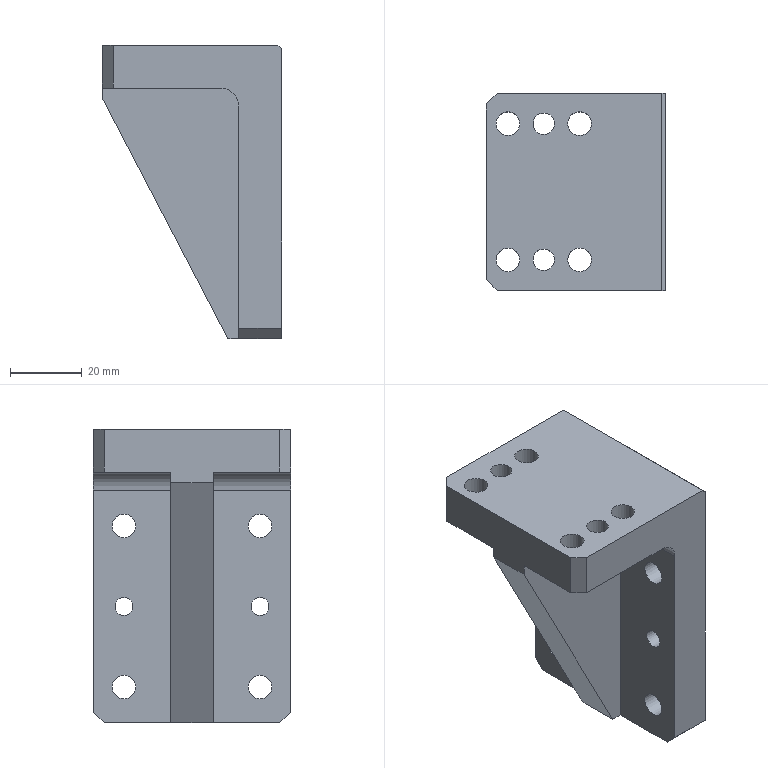Part | NX | 1 solid | 32 faces | box 50 x 55 x 82 mm | volume 92603 mm3 | plane 18 | cylinder 14 | commonest cylinder face diameters 6.6 x8 5 x2 6 x2 10 x2
STEP:
#1=CARTESIAN_POINT('',(24.,55.,41.));
#2=VERTEX_POINT('',#1);
#3=CARTESIAN_POINT('',(25.,55.,40.));
#4=VERTEX_POINT('',#3);
#5=CARTESIAN_POINT('',(25.,55.,40.));
#6=DIRECTION('',(0.7071,0.,-0.7071));
#7=VECTOR('',#6,1000.);
#8=LINE('',#5,#7);
#9=EDGE_CURVE('',#2,#4,#8,.T.);
#10=ORIENTED_EDGE('',*,*,#9,.F.);
#11=CARTESIAN_POINT('',(24.,0.,41.));
#12=VERTEX_POINT('',#11);
#13=CARTESIAN_POINT('',(24.,55.,41.));
#14=DIRECTION('',(0.,1.,0.));
#15=VECTOR('',#14,1000.);
#16=LINE('',#13,#15);
#17=EDGE_CURVE('',#12,#2,#16,.T.);
#18=ORIENTED_EDGE('',*,*,#17,.F.);
#19=CARTESIAN_POINT('',(25.,0.,40.));
#20=VERTEX_POINT('',#19);
#21=CARTESIAN_POINT('',(32.5,0.,32.5));
#22=DIRECTION('',(-0.7071,0.,0.7071));
#23=VECTOR('',#22,1000.);
#24=LINE('',#21,#23);
#25=EDGE_CURVE('',#20,#12,#24,.T.);
#26=ORIENTED_EDGE('',*,*,#25,.F.);
#27=CARTESIAN_POINT('',(25.,55.,40.));
#28=DIRECTION('',(0.,-1.,0.));
#29=VECTOR('',#28,1000.);
#30=LINE('',#27,#29);
#31=EDGE_CURVE('',#4,#20,#30,.T.);
#32=ORIENTED_EDGE('',*,*,#31,.F.);
#33=EDGE_LOOP('',(#10,#18,#26,#32));
#34=FACE_BOUND('',#33,.T.);
#35=CARTESIAN_POINT('',(25.,55.,40.));
#36=DIRECTION('',(-0.7071,0.,-0.7071));
#37=DIRECTION('',(0.,-1.,0.));
#38=AXIS2_PLACEMENT_3D('',#35,#36,#37);
#39=PLANE('',#38);
#40=ADVANCED_FACE('',(#34),#39,.F.);
#41=CARTESIAN_POINT('',(25.,52.,-41.));
#42=VERTEX_POINT('',#41);
#43=CARTESIAN_POINT('',(25.,55.,-38.));
#44=VERTEX_POINT('',#43);
#45=CARTESIAN_POINT('',(25.,55.,-38.));
#46=DIRECTION('',(0.,0.7071,0.7071));
#47=VECTOR('',#46,1000.);
#48=LINE('',#45,#47);
#49=EDGE_CURVE('',#42,#44,#48,.T.);
#50=ORIENTED_EDGE('',*,*,#49,.F.);
#51=CARTESIAN_POINT('',(13.,52.,-41.));
#52=VERTEX_POINT('',#51);
#53=CARTESIAN_POINT('',(-25.,52.,-41.));
#54=DIRECTION('',(1.,0.,0.));
#55=VECTOR('',#54,1000.);
#56=LINE('',#53,#55);
#57=EDGE_CURVE('',#52,#42,#56,.T.);
#58=ORIENTED_EDGE('',*,*,#57,.F.);
#59=CARTESIAN_POINT('',(13.,55.,-38.));
#60=VERTEX_POINT('',#59);
#61=CARTESIAN_POINT('',(13.,36.75,-56.25));
#62=DIRECTION('',(0.,-0.7071,-0.7071));
#63=VECTOR('',#62,1000.);
#64=LINE('',#61,#63);
#65=EDGE_CURVE('',#60,#52,#64,.T.);
#66=ORIENTED_EDGE('',*,*,#65,.F.);
#67=CARTESIAN_POINT('',(0.,55.,-38.));
#68=DIRECTION('',(-1.,0.,0.));
#69=VECTOR('',#68,1000.);
#70=LINE('',#67,#69);
#71=EDGE_CURVE('',#44,#60,#70,.T.);
#72=ORIENTED_EDGE('',*,*,#71,.F.);
#73=EDGE_LOOP('',(#50,#58,#66,#72));
#74=FACE_BOUND('',#73,.T.);
#75=CARTESIAN_POINT('',(0.,55.,-38.));
#76=DIRECTION('',(0.,-0.7071,0.7071));
#77=DIRECTION('',(-1.,0.,0.));
#78=AXIS2_PLACEMENT_3D('',#75,#76,#77);
#79=PLANE('',#78);
#80=ADVANCED_FACE('',(#74),#79,.F.);
#81=CARTESIAN_POINT('',(-25.,52.,29.));
#82=VERTEX_POINT('',#81);
#83=CARTESIAN_POINT('',(-22.,55.,29.));
#84=VERTEX_POINT('',#83);
#85=CARTESIAN_POINT('',(-21.25,55.75,29.));
#86=DIRECTION('',(0.7071,0.7071,0.));
#87=VECTOR('',#86,1000.);
#88=LINE('',#85,#87);
#89=EDGE_CURVE('',#82,#84,#88,.T.);
#90=ORIENTED_EDGE('',*,*,#89,.F.);
#91=CARTESIAN_POINT('',(-25.,52.,41.));
#92=VERTEX_POINT('',#91);
#93=CARTESIAN_POINT('',(-25.,52.,41.));
#94=DIRECTION('',(0.,0.,-1.));
#95=VECTOR('',#94,1000.);
#96=LINE('',#93,#95);
#97=EDGE_CURVE('',#92,#82,#96,.T.);
#98=ORIENTED_EDGE('',*,*,#97,.F.);
#99=CARTESIAN_POINT('',(-22.,55.,41.));
#100=VERTEX_POINT('',#99);
#101=CARTESIAN_POINT('',(-22.,55.,41.));
#102=DIRECTION('',(-0.7071,-0.7071,0.));
#103=VECTOR('',#102,1000.);
#104=LINE('',#101,#103);
#105=EDGE_CURVE('',#100,#92,#104,.T.);
#106=ORIENTED_EDGE('',*,*,#105,.F.);
#107=CARTESIAN_POINT('',(-22.,55.,0.));
#108=DIRECTION('',(0.,0.,1.));
#109=VECTOR('',#108,1000.);
#110=LINE('',#107,#109);
#111=EDGE_CURVE('',#84,#100,#110,.T.);
#112=ORIENTED_EDGE('',*,*,#111,.F.);
#113=EDGE_LOOP('',(#90,#98,#106,#112));
#114=FACE_BOUND('',#113,.T.);
#115=CARTESIAN_POINT('',(-22.,55.,0.));
#116=DIRECTION('',(0.7071,-0.7071,0.));
#117=DIRECTION('',(0.,0.,1.));
#118=AXIS2_PLACEMENT_3D('',#115,#116,#117);
#119=PLANE('',#118);
#120=ADVANCED_FACE('',(#114),#119,.F.);
#121=CARTESIAN_POINT('',(25.,0.,-38.));
#122=VERTEX_POINT('',#121);
#123=CARTESIAN_POINT('',(25.,3.,-41.));
#124=VERTEX_POINT('',#123);
#125=CARTESIAN_POINT('',(25.,3.,-41.));
#126=DIRECTION('',(0.,0.7071,-0.7071));
#127=VECTOR('',#126,1000.);
#128=LINE('',#125,#127);
#129=EDGE_CURVE('',#122,#124,#128,.T.);
#130=ORIENTED_EDGE('',*,*,#129,.F.);
#131=CARTESIAN_POINT('',(13.,0.,-38.));
#132=VERTEX_POINT('',#131);
#133=CARTESIAN_POINT('',(25.,0.,-38.));
#134=DIRECTION('',(1.,0.,0.));
#135=VECTOR('',#134,1000.);
#136=LINE('',#133,#135);
#137=EDGE_CURVE('',#132,#122,#136,.T.);
#138=ORIENTED_EDGE('',*,*,#137,.F.);
#139=CARTESIAN_POINT('',(13.,3.,-41.));
#140=VERTEX_POINT('',#139);
#141=CARTESIAN_POINT('',(13.,12.25,-50.25));
#142=DIRECTION('',(0.,-0.7071,0.7071));
#143=VECTOR('',#142,1000.);
#144=LINE('',#141,#143);
#145=EDGE_CURVE('',#140,#132,#144,.T.);
#146=ORIENTED_EDGE('',*,*,#145,.F.);
#147=CARTESIAN_POINT('',(13.,3.,-41.));
#148=DIRECTION('',(-1.,0.,0.));
#149=VECTOR('',#148,1000.);
#150=LINE('',#147,#149);
#151=EDGE_CURVE('',#124,#140,#150,.T.);
#152=ORIENTED_EDGE('',*,*,#151,.F.);
#153=EDGE_LOOP('',(#130,#138,#146,#152));
#154=FACE_BOUND('',#153,.T.);
#155=CARTESIAN_POINT('',(-25.,3.,-41.));
#156=DIRECTION('',(0.,-0.7071,-0.7071));
#157=DIRECTION('',(1.,0.,0.));
#158=AXIS2_PLACEMENT_3D('',#155,#156,#157);
#159=PLANE('',#158);
#160=ADVANCED_FACE('',(#154),#159,.T.);
#161=CARTESIAN_POINT('',(-22.,0.,29.));
#162=VERTEX_POINT('',#161);
#163=CARTESIAN_POINT('',(-25.,3.,29.));
#164=VERTEX_POINT('',#163);
#165=CARTESIAN_POINT('',(-15.25,-6.75,29.));
#166=DIRECTION('',(-0.7071,0.7071,0.));
#167=VECTOR('',#166,1000.);
#168=LINE('',#165,#167);
#169=EDGE_CURVE('',#162,#164,#168,.T.);
#170=ORIENTED_EDGE('',*,*,#169,.F.);
#171=CARTESIAN_POINT('',(-22.,0.,41.));
#172=VERTEX_POINT('',#171);
#173=CARTESIAN_POINT('',(-22.,0.,29.));
#174=DIRECTION('',(0.,0.,-1.));
#175=VECTOR('',#174,1000.);
#176=LINE('',#173,#175);
#177=EDGE_CURVE('',#172,#162,#176,.T.);
#178=ORIENTED_EDGE('',*,*,#177,.F.);
#179=CARTESIAN_POINT('',(-25.,3.,41.));
#180=VERTEX_POINT('',#179);
#181=CARTESIAN_POINT('',(-25.,3.,41.));
#182=DIRECTION('',(0.7071,-0.7071,0.));
#183=VECTOR('',#182,1000.);
#184=LINE('',#181,#183);
#185=EDGE_CURVE('',#180,#172,#184,.T.);
#186=ORIENTED_EDGE('',*,*,#185,.F.);
#187=CARTESIAN_POINT('',(-25.,3.,41.));
#188=DIRECTION('',(0.,0.,1.));
#189=VECTOR('',#188,1000.);
#190=LINE('',#187,#189);
#191=EDGE_CURVE('',#164,#180,#190,.T.);
#192=ORIENTED_EDGE('',*,*,#191,.F.);
#193=EDGE_LOOP('',(#170,#178,#186,#192));
#194=FACE_BOUND('',#193,.T.);
#195=CARTESIAN_POINT('',(-25.,3.,41.));
#196=DIRECTION('',(-0.7071,-0.7071,0.));
#197=DIRECTION('',(0.,0.,-1.));
#198=AXIS2_PLACEMENT_3D('',#195,#196,#197);
#199=PLANE('',#198);
#200=ADVANCED_FACE('',(#194),#199,.T.);
#201=CARTESIAN_POINT('',(8.,33.5,29.));
#202=VERTEX_POINT('',#201);
#203=CARTESIAN_POINT('',(13.,33.5,24.));
#204=VERTEX_POINT('',#203);
#205=CARTESIAN_POINT('',(8.,33.5,24.));
#206=DIRECTION('',(0.,1.,0.));
#207=DIRECTION('',(0.,0.,1.));
#208=AXIS2_PLACEMENT_3D('',#205,#206,#207);
#209=CIRCLE('',#208,5.);
#210=EDGE_CURVE('',#202,#204,#209,.T.);
#211=ORIENTED_EDGE('',*,*,#210,.F.);
#212=CARTESIAN_POINT('',(8.,55.,29.));
#213=VERTEX_POINT('',#212);
#214=CARTESIAN_POINT('',(8.,33.5,29.));
#215=DIRECTION('',(0.,-1.,0.));
#216=VECTOR('',#215,1000.);
#217=LINE('',#214,#216);
#218=EDGE_CURVE('',#213,#202,#217,.T.);
#219=ORIENTED_EDGE('',*,*,#218,.F.);
#220=CARTESIAN_POINT('',(13.,55.,24.));
#221=VERTEX_POINT('',#220);
#222=CARTESIAN_POINT('',(8.,55.,24.));
#223=DIRECTION('',(0.,-1.,0.));
#224=DIRECTION('',(0.,0.,-1.));
#225=AXIS2_PLACEMENT_3D('',#222,#223,#224);
#226=CIRCLE('',#225,5.);
#227=EDGE_CURVE('',#221,#213,#226,.T.);
#228=ORIENTED_EDGE('',*,*,#227,.F.);
#229=CARTESIAN_POINT('',(13.,33.5,24.));
#230=DIRECTION('',(0.,1.,0.));
#231=VECTOR('',#230,1000.);
#232=LINE('',#229,#231);
#233=EDGE_CURVE('',#204,#221,#232,.T.);
#234=ORIENTED_EDGE('',*,*,#233,.F.);
#235=EDGE_LOOP('',(#211,#219,#228,#234));
#236=FACE_BOUND('',#235,.T.);
#237=CARTESIAN_POINT('',(8.,33.5,24.));
#238=DIRECTION('',(0.,-1.,0.));
#239=DIRECTION('',(0.,0.,-1.));
#240=AXIS2_PLACEMENT_3D('',#237,#238,#239);
#241=CYLINDRICAL_SURFACE('',#240,5.);
#242=ADVANCED_FACE('',(#236),#241,.F.);
#243=CARTESIAN_POINT('',(13.,21.5,24.));
#244=VERTEX_POINT('',#243);
#245=CARTESIAN_POINT('',(8.,21.5,29.));
#246=VERTEX_POINT('',#245);
#247=CARTESIAN_POINT('',(8.,21.5,24.));
#248=DIRECTION('',(0.,-1.,0.));
#249=DIRECTION('',(0.,0.,-1.));
#250=AXIS2_PLACEMENT_3D('',#247,#248,#249);
#251=CIRCLE('',#250,5.);
#252=EDGE_CURVE('',#244,#246,#251,.T.);
#253=ORIENTED_EDGE('',*,*,#252,.F.);
#254=CARTESIAN_POINT('',(13.,0.,24.));
#255=VERTEX_POINT('',#254);
#256=CARTESIAN_POINT('',(13.,21.5,24.));
#257=DIRECTION('',(0.,1.,0.));
#258=VECTOR('',#257,1000.);
#259=LINE('',#256,#258);
#260=EDGE_CURVE('',#255,#244,#259,.T.);
#261=ORIENTED_EDGE('',*,*,#260,.F.);
#262=CARTESIAN_POINT('',(8.,0.,29.));
#263=VERTEX_POINT('',#262);
#264=CARTESIAN_POINT('',(8.,0.,24.));
#265=DIRECTION('',(0.,1.,0.));
#266=DIRECTION('',(0.,0.,-1.));
#267=AXIS2_PLACEMENT_3D('',#264,#265,#266);
#268=CIRCLE('',#267,5.);
#269=EDGE_CURVE('',#263,#255,#268,.T.);
#270=ORIENTED_EDGE('',*,*,#269,.F.);
#271=CARTESIAN_POINT('',(8.,0.,29.));
#272=DIRECTION('',(0.,-1.,0.));
#273=VECTOR('',#272,1000.);
#274=LINE('',#271,#273);
#275=EDGE_CURVE('',#246,#263,#274,.T.);
#276=ORIENTED_EDGE('',*,*,#275,.F.);
#277=EDGE_LOOP('',(#253,#261,#270,#276));
#278=FACE_BOUND('',#277,.T.);
#279=CARTESIAN_POINT('',(8.,21.5,24.));
#280=DIRECTION('',(0.,1.,0.));
#281=DIRECTION('',(0.,0.,1.));
#282=AXIS2_PLACEMENT_3D('',#279,#280,#281);
#283=CYLINDRICAL_SURFACE('',#282,5.);
#284=ADVANCED_FACE('',(#278),#283,.F.);
#285=CARTESIAN_POINT('',(13.,21.5,-41.));
#286=VERTEX_POINT('',#285);
#287=CARTESIAN_POINT('',(13.,21.5,-41.));
#288=DIRECTION('',(0.,0.,-1.));
#289=VECTOR('',#288,1000.);
#290=LINE('',#287,#289);
#291=EDGE_CURVE('',#244,#286,#290,.T.);
#292=ORIENTED_EDGE('',*,*,#291,.F.);
#293=ORIENTED_EDGE('',*,*,#252,.T.);
#294=CARTESIAN_POINT('',(-25.,21.5,29.));
#295=VERTEX_POINT('',#294);
#296=CARTESIAN_POINT('',(13.,21.5,29.));
#297=DIRECTION('',(1.,0.,0.));
#298=VECTOR('',#297,1000.);
#299=LINE('',#296,#298);
#300=EDGE_CURVE('',#295,#246,#299,.T.);
#301=ORIENTED_EDGE('',*,*,#300,.F.);
#302=CARTESIAN_POINT('',(-25.,21.5,26.));
#303=VERTEX_POINT('',#302);
#304=CARTESIAN_POINT('',(-25.,21.5,26.));
#305=DIRECTION('',(0.,0.,1.));
#306=VECTOR('',#305,1000.);
#307=LINE('',#304,#306);
#308=EDGE_CURVE('',#303,#295,#307,.T.);
#309=ORIENTED_EDGE('',*,*,#308,.F.);
#310=CARTESIAN_POINT('',(10.,21.5,-41.));
#311=VERTEX_POINT('',#310);
#312=CARTESIAN_POINT('',(-25.,21.5,26.));
#313=DIRECTION('',(-0.463,0.,0.8863));
#314=VECTOR('',#313,1000.);
#315=LINE('',#312,#314);
#316=EDGE_CURVE('',#311,#303,#315,.T.);
#317=ORIENTED_EDGE('',*,*,#316,.F.);
#318=CARTESIAN_POINT('',(13.,21.5,-41.));
#319=DIRECTION('',(-1.,0.,0.));
#320=VECTOR('',#319,1000.);
#321=LINE('',#318,#320);
#322=EDGE_CURVE('',#286,#311,#321,.T.);
#323=ORIENTED_EDGE('',*,*,#322,.F.);
#324=EDGE_LOOP('',(#292,#293,#301,#309,#317,#323));
#325=FACE_BOUND('',#324,.T.);
#326=CARTESIAN_POINT('',(0.,21.5,0.));
#327=DIRECTION('',(0.,-1.,0.));
#328=DIRECTION('',(0.,0.,1.));
#329=AXIS2_PLACEMENT_3D('',#326,#327,#328);
#330=PLANE('',#329);
#331=ADVANCED_FACE('',(#325),#330,.T.);
#332=CARTESIAN_POINT('',(13.,21.5,-41.));
#333=DIRECTION('',(0.,-1.,0.));
#334=VECTOR('',#333,1000.);
#335=LINE('',#332,#334);
#336=EDGE_CURVE('',#286,#140,#335,.T.);
#337=ORIENTED_EDGE('',*,*,#336,.T.);
#338=ORIENTED_EDGE('',*,*,#145,.T.);
#339=CARTESIAN_POINT('',(13.,0.,-41.));
#340=DIRECTION('',(0.,0.,-1.));
#341=VECTOR('',#340,1000.);
#342=LINE('',#339,#341);
#343=EDGE_CURVE('',#255,#132,#342,.T.);
#344=ORIENTED_EDGE('',*,*,#343,.F.);
#345=ORIENTED_EDGE('',*,*,#260,.T.);
#346=ORIENTED_EDGE('',*,*,#291,.T.);
#347=EDGE_LOOP('',(#337,#338,#344,#345,#346));
#348=FACE_BOUND('',#347,.T.);
#349=CARTESIAN_POINT('',(13.,8.5,17.3));
#350=VERTEX_POINT('',#349);
#351=CARTESIAN_POINT('',(13.,8.5,14.));
#352=DIRECTION('',(-1.,0.,0.));
#353=DIRECTION('',(0.,0.,1.));
#354=AXIS2_PLACEMENT_3D('',#351,#352,#353);
#355=CIRCLE('',#354,3.3);
#356=EDGE_CURVE('',#350,#350,#355,.T.);
#357=ORIENTED_EDGE('',*,*,#356,.F.);
#358=EDGE_LOOP('',(#357));
#359=FACE_BOUND('',#358,.T.);
#360=CARTESIAN_POINT('',(13.,8.5,-27.7));
#361=VERTEX_POINT('',#360);
#362=CARTESIAN_POINT('',(13.,8.5,-31.));
#363=DIRECTION('',(-1.,0.,0.));
#364=DIRECTION('',(0.,0.,1.));
#365=AXIS2_PLACEMENT_3D('',#362,#363,#364);
#366=CIRCLE('',#365,3.3);
#367=EDGE_CURVE('',#361,#361,#366,.T.);
#368=ORIENTED_EDGE('',*,*,#367,.F.);
#369=EDGE_LOOP('',(#368));
#370=FACE_BOUND('',#369,.T.);
#371=CARTESIAN_POINT('',(13.,8.5,-6.));
#372=VERTEX_POINT('',#371);
#373=CARTESIAN_POINT('',(13.,8.5,-8.5));
#374=DIRECTION('',(-1.,0.,0.));
#375=DIRECTION('',(0.,0.,1.));
#376=AXIS2_PLACEMENT_3D('',#373,#374,#375);
#377=CIRCLE('',#376,2.5);
#378=EDGE_CURVE('',#372,#372,#377,.T.);
#379=ORIENTED_EDGE('',*,*,#378,.F.);
#380=EDGE_LOOP('',(#379));
#381=FACE_BOUND('',#380,.T.);
#382=CARTESIAN_POINT('',(13.,21.5,-41.));
#383=DIRECTION('',(-1.,0.,0.));
#384=DIRECTION('',(0.,0.,1.));
#385=AXIS2_PLACEMENT_3D('',#382,#383,#384);
#386=PLANE('',#385);
#387=ADVANCED_FACE('',(#348,#359,#370,#381),#386,.T.);
#388=CARTESIAN_POINT('',(13.,0.,29.));
#389=DIRECTION('',(1.,0.,0.));
#390=VECTOR('',#389,1000.);
#391=LINE('',#388,#390);
#392=EDGE_CURVE('',#162,#263,#391,.T.);
#393=ORIENTED_EDGE('',*,*,#392,.F.);
#394=ORIENTED_EDGE('',*,*,#169,.T.);
#395=CARTESIAN_POINT('',(-25.,21.5,29.));
#396=DIRECTION('',(0.,-1.,0.));
#397=VECTOR('',#396,1000.);
#398=LINE('',#395,#397);
#399=EDGE_CURVE('',#295,#164,#398,.T.);
#400=ORIENTED_EDGE('',*,*,#399,.F.);
#401=ORIENTED_EDGE('',*,*,#300,.T.);
#402=ORIENTED_EDGE('',*,*,#275,.T.);
#403=EDGE_LOOP('',(#393,#394,#400,#401,#402));
#404=FACE_BOUND('',#403,.T.);
#405=CARTESIAN_POINT('',(-22.3,8.5,29.));
#406=VERTEX_POINT('',#405);
#407=CARTESIAN_POINT('',(-19.,8.5,29.));
#408=DIRECTION('',(0.,0.,-1.));
#409=DIRECTION('',(-1.,0.,0.));
#410=AXIS2_PLACEMENT_3D('',#407,#408,#409);
#411=CIRCLE('',#410,3.3);
#412=EDGE_CURVE('',#406,#406,#411,.T.);
#413=ORIENTED_EDGE('',*,*,#412,.F.);
#414=EDGE_LOOP('',(#413));
#415=FACE_BOUND('',#414,.T.);
#416=CARTESIAN_POINT('',(-2.3,8.5,29.));
#417=VERTEX_POINT('',#416);
#418=CARTESIAN_POINT('',(1.,8.5,29.));
#419=DIRECTION('',(0.,0.,-1.));
#420=DIRECTION('',(-1.,0.,0.));
#421=AXIS2_PLACEMENT_3D('',#418,#419,#420);
#422=CIRCLE('',#421,3.3);
#423=EDGE_CURVE('',#417,#417,#422,.T.);
#424=ORIENTED_EDGE('',*,*,#423,.F.);
#425=EDGE_LOOP('',(#424));
#426=FACE_BOUND('',#425,.T.);
#427=CARTESIAN_POINT('',(-12.,8.5,29.));
#428=VERTEX_POINT('',#427);
#429=CARTESIAN_POINT('',(-9.,8.5,29.));
#430=DIRECTION('',(0.,0.,-1.));
#431=DIRECTION('',(-1.,0.,0.));
#432=AXIS2_PLACEMENT_3D('',#429,#430,#431);
#433=CIRCLE('',#432,3.);
#434=EDGE_CURVE('',#428,#428,#433,.T.);
#435=ORIENTED_EDGE('',*,*,#434,.F.);
#436=EDGE_LOOP('',(#435));
#437=FACE_BOUND('',#436,.T.);
#438=CARTESIAN_POINT('',(13.,21.5,29.));
#439=DIRECTION('',(0.,0.,-1.));
#440=DIRECTION('',(-1.,0.,0.));
#441=AXIS2_PLACEMENT_3D('',#438,#439,#440);
#442=PLANE('',#441);
#443=ADVANCED_FACE('',(#404,#415,#426,#437),#442,.T.);
#444=CARTESIAN_POINT('',(-25.,33.5,29.));
#445=VERTEX_POINT('',#444);
#446=CARTESIAN_POINT('',(0.,33.5,29.));
#447=DIRECTION('',(1.,0.,0.));
#448=VECTOR('',#447,1000.);
#449=LINE('',#446,#448);
#450=EDGE_CURVE('',#445,#202,#449,.T.);
#451=ORIENTED_EDGE('',*,*,#450,.T.);
#452=ORIENTED_EDGE('',*,*,#210,.T.);
#453=CARTESIAN_POINT('',(13.,33.5,-41.));
#454=VERTEX_POINT('',#453);
#455=CARTESIAN_POINT('',(13.,33.5,0.));
#456=DIRECTION('',(0.,0.,-1.));
#457=VECTOR('',#456,1000.);
#458=LINE('',#455,#457);
#459=EDGE_CURVE('',#204,#454,#458,.T.);
#460=ORIENTED_EDGE('',*,*,#459,.T.);
#461=CARTESIAN_POINT('',(10.,33.5,-41.));
#462=VERTEX_POINT('',#461);
#463=CARTESIAN_POINT('',(13.,33.5,-41.));
#464=DIRECTION('',(-1.,0.,0.));
#465=VECTOR('',#464,1000.);
#466=LINE('',#463,#465);
#467=EDGE_CURVE('',#454,#462,#466,.T.);
#468=ORIENTED_EDGE('',*,*,#467,.T.);
#469=CARTESIAN_POINT('',(-25.,33.5,26.));
#470=VERTEX_POINT('',#469);
#471=CARTESIAN_POINT('',(-25.,33.5,26.));
#472=DIRECTION('',(-0.463,0.,0.8863));
#473=VECTOR('',#472,1000.);
#474=LINE('',#471,#473);
#475=EDGE_CURVE('',#462,#470,#474,.T.);
#476=ORIENTED_EDGE('',*,*,#475,.T.);
#477=CARTESIAN_POINT('',(-25.,33.5,26.));
#478=DIRECTION('',(0.,0.,1.));
#479=VECTOR('',#478,1000.);
#480=LINE('',#477,#479);
#481=EDGE_CURVE('',#470,#445,#480,.T.);
#482=ORIENTED_EDGE('',*,*,#481,.T.);
#483=EDGE_LOOP('',(#451,#452,#460,#468,#476,#482));
#484=FACE_BOUND('',#483,.T.);
#485=CARTESIAN_POINT('',(0.,33.5,0.));
#486=DIRECTION('',(0.,1.,0.));
#487=DIRECTION('',(0.,0.,1.));
#488=AXIS2_PLACEMENT_3D('',#485,#486,#487);
#489=PLANE('',#488);
#490=ADVANCED_FACE('',(#484),#489,.T.);
#491=CARTESIAN_POINT('',(13.,55.,-41.));
#492=DIRECTION('',(0.,0.,-1.));
#493=VECTOR('',#492,1000.);
#494=LINE('',#491,#493);
#495=EDGE_CURVE('',#221,#60,#494,.T.);
#496=ORIENTED_EDGE('',*,*,#495,.T.);
#497=ORIENTED_EDGE('',*,*,#65,.T.);
#498=CARTESIAN_POINT('',(13.,55.,-41.));
#499=DIRECTION('',(0.,1.,0.));
#500=VECTOR('',#499,1000.);
#501=LINE('',#498,#500);
#502=EDGE_CURVE('',#454,#52,#501,.T.);
#503=ORIENTED_EDGE('',*,*,#502,.F.);
#504=ORIENTED_EDGE('',*,*,#459,.F.);
#505=ORIENTED_EDGE('',*,*,#233,.T.);
#506=EDGE_LOOP('',(#496,#497,#503,#504,#505));
#507=FACE_BOUND('',#506,.T.);
#508=CARTESIAN_POINT('',(13.,46.5,17.3));
#509=VERTEX_POINT('',#508);
#510=CARTESIAN_POINT('',(13.,46.5,14.));
#511=DIRECTION('',(-1.,0.,0.));
#512=DIRECTION('',(0.,0.,1.));
#513=AXIS2_PLACEMENT_3D('',#510,#511,#512);
#514=CIRCLE('',#513,3.3);
#515=EDGE_CURVE('',#509,#509,#514,.T.);
#516=ORIENTED_EDGE('',*,*,#515,.F.);
#517=EDGE_LOOP('',(#516));
#518=FACE_BOUND('',#517,.T.);
#519=CARTESIAN_POINT('',(13.,46.5,-27.7));
#520=VERTEX_POINT('',#519);
#521=CARTESIAN_POINT('',(13.,46.5,-31.));
#522=DIRECTION('',(-1.,0.,0.));
#523=DIRECTION('',(0.,0.,1.));
#524=AXIS2_PLACEMENT_3D('',#521,#522,#523);
#525=CIRCLE('',#524,3.3);
#526=EDGE_CURVE('',#520,#520,#525,.T.);
#527=ORIENTED_EDGE('',*,*,#526,.F.);
#528=EDGE_LOOP('',(#527));
#529=FACE_BOUND('',#528,.T.);
#530=CARTESIAN_POINT('',(13.,46.5,-6.));
#531=VERTEX_POINT('',#530);
#532=CARTESIAN_POINT('',(13.,46.5,-8.5));
#533=DIRECTION('',(-1.,0.,0.));
#534=DIRECTION('',(0.,0.,1.));
#535=AXIS2_PLACEMENT_3D('',#532,#533,#534);
#536=CIRCLE('',#535,2.5);
#537=EDGE_CURVE('',#531,#531,#536,.T.);
#538=ORIENTED_EDGE('',*,*,#537,.F.);
#539=EDGE_LOOP('',(#538));
#540=FACE_BOUND('',#539,.T.);
#541=CARTESIAN_POINT('',(13.,21.5,-41.));
#542=DIRECTION('',(-1.,0.,0.));
#543=DIRECTION('',(0.,0.,1.));
#544=AXIS2_PLACEMENT_3D('',#541,#542,#543);
#545=PLANE('',#544);
#546=ADVANCED_FACE('',(#507,#518,#529,#540),#545,.T.);
#547=CARTESIAN_POINT('',(-25.,55.,41.));
#548=DIRECTION('',(1.,0.,0.));
#549=VECTOR('',#548,1000.);
#550=LINE('',#547,#549);
#551=EDGE_CURVE('',#100,#2,#550,.T.);
#552=ORIENTED_EDGE('',*,*,#551,.T.);
#553=ORIENTED_EDGE('',*,*,#9,.T.);
#554=CARTESIAN_POINT('',(25.,55.,41.));
#555=DIRECTION('',(0.,0.,-1.));
#556=VECTOR('',#555,1000.);
#557=LINE('',#554,#556);
#558=EDGE_CURVE('',#4,#44,#557,.T.);
#559=ORIENTED_EDGE('',*,*,#558,.T.);
#560=ORIENTED_EDGE('',*,*,#71,.T.);
#561=ORIENTED_EDGE('',*,*,#495,.F.);
#562=ORIENTED_EDGE('',*,*,#227,.T.);
#563=CARTESIAN_POINT('',(13.,55.,29.));
#564=DIRECTION('',(1.,0.,0.));
#565=VECTOR('',#564,1000.);
#566=LINE('',#563,#565);
#567=EDGE_CURVE('',#84,#213,#566,.T.);
#568=ORIENTED_EDGE('',*,*,#567,.F.);
#569=ORIENTED_EDGE('',*,*,#111,.T.);
#570=EDGE_LOOP('',(#552,#553,#559,#560,#561,#562,#568,#569));
#571=FACE_BOUND('',#570,.T.);
#572=CARTESIAN_POINT('',(0.,55.,0.));
#573=DIRECTION('',(0.,-1.,0.));
#574=DIRECTION('',(0.,0.,-1.));
#575=AXIS2_PLACEMENT_3D('',#572,#573,#574);
#576=PLANE('',#575);
#577=ADVANCED_FACE('',(#571),#576,.F.);
#578=CARTESIAN_POINT('',(-25.,0.,41.));
#579=DIRECTION('',(1.,0.,0.));
#580=VECTOR('',#579,1000.);
#581=LINE('',#578,#580);
#582=EDGE_CURVE('',#172,#12,#581,.T.);
#583=ORIENTED_EDGE('',*,*,#582,.T.);
#584=ORIENTED_EDGE('',*,*,#17,.T.);
#585=ORIENTED_EDGE('',*,*,#551,.F.);
#586=ORIENTED_EDGE('',*,*,#105,.T.);
#587=CARTESIAN_POINT('',(-25.,55.,41.));
#588=DIRECTION('',(0.,-1.,0.));
#589=VECTOR('',#588,1000.);
#590=LINE('',#587,#589);
#591=EDGE_CURVE('',#92,#180,#590,.T.);
#592=ORIENTED_EDGE('',*,*,#591,.T.);
#593=ORIENTED_EDGE('',*,*,#185,.T.);
#594=EDGE_LOOP('',(#583,#584,#585,#586,#592,#593));
#595=FACE_BOUND('',#594,.T.);
#596=CARTESIAN_POINT('',(-22.3,46.5,41.));
#597=VERTEX_POINT('',#596);
#598=CARTESIAN_POINT('',(-19.,46.5,41.));
#599=DIRECTION('',(0.,0.,-1.));
#600=DIRECTION('',(-1.,0.,0.));
#601=AXIS2_PLACEMENT_3D('',#598,#599,#600);
#602=CIRCLE('',#601,3.3);
#603=EDGE_CURVE('',#597,#597,#602,.T.);
#604=ORIENTED_EDGE('',*,*,#603,.T.);
#605=EDGE_LOOP('',(#604));
#606=FACE_BOUND('',#605,.T.);
#607=CARTESIAN_POINT('',(-2.3,46.5,41.));
#608=VERTEX_POINT('',#607);
#609=CARTESIAN_POINT('',(1.,46.5,41.));
#610=DIRECTION('',(0.,0.,-1.));
#611=DIRECTION('',(-1.,0.,0.));
#612=AXIS2_PLACEMENT_3D('',#609,#610,#611);
#613=CIRCLE('',#612,3.3);
#614=EDGE_CURVE('',#608,#608,#613,.T.);
#615=ORIENTED_EDGE('',*,*,#614,.T.);
#616=EDGE_LOOP('',(#615));
#617=FACE_BOUND('',#616,.T.);
#618=CARTESIAN_POINT('',(-22.3,8.5,41.));
#619=VERTEX_POINT('',#618);
#620=CARTESIAN_POINT('',(-19.,8.5,41.));
#621=DIRECTION('',(0.,0.,-1.));
#622=DIRECTION('',(-1.,0.,0.));
#623=AXIS2_PLACEMENT_3D('',#620,#621,#622);
#624=CIRCLE('',#623,3.3);
#625=EDGE_CURVE('',#619,#619,#624,.T.);
#626=ORIENTED_EDGE('',*,*,#625,.T.);
#627=EDGE_LOOP('',(#626));
#628=FACE_BOUND('',#627,.T.);
#629=CARTESIAN_POINT('',(-2.3,8.5,41.));
#630=VERTEX_POINT('',#629);
#631=CARTESIAN_POINT('',(1.,8.5,41.));
#632=DIRECTION('',(0.,0.,-1.));
#633=DIRECTION('',(-1.,0.,0.));
#634=AXIS2_PLACEMENT_3D('',#631,#632,#633);
#635=CIRCLE('',#634,3.3);
#636=EDGE_CURVE('',#630,#630,#635,.T.);
#637=ORIENTED_EDGE('',*,*,#636,.T.);
#638=EDGE_LOOP('',(#637));
#639=FACE_BOUND('',#638,.T.);
#640=CARTESIAN_POINT('',(-12.,46.5,41.));
#641=VERTEX_POINT('',#640);
#642=CARTESIAN_POINT('',(-9.,46.5,41.));
#643=DIRECTION('',(0.,0.,-1.));
#644=DIRECTION('',(-1.,0.,0.));
#645=AXIS2_PLACEMENT_3D('',#642,#643,#644);
#646=CIRCLE('',#645,3.);
#647=EDGE_CURVE('',#641,#641,#646,.T.);
#648=ORIENTED_EDGE('',*,*,#647,.T.);
#649=EDGE_LOOP('',(#648));
#650=FACE_BOUND('',#649,.T.);
#651=CARTESIAN_POINT('',(-12.,8.5,41.));
#652=VERTEX_POINT('',#651);
#653=CARTESIAN_POINT('',(-9.,8.5,41.));
#654=DIRECTION('',(0.,0.,-1.));
#655=DIRECTION('',(-1.,0.,0.));
#656=AXIS2_PLACEMENT_3D('',#653,#654,#655);
#657=CIRCLE('',#656,3.);
#658=EDGE_CURVE('',#652,#652,#657,.T.);
#659=ORIENTED_EDGE('',*,*,#658,.T.);
#660=EDGE_LOOP('',(#659));
#661=FACE_BOUND('',#660,.T.);
#662=CARTESIAN_POINT('',(-25.,55.,41.));
#663=DIRECTION('',(0.,0.,-1.));
#664=DIRECTION('',(-1.,0.,0.));
#665=AXIS2_PLACEMENT_3D('',#662,#663,#664);
#666=PLANE('',#665);
#667=ADVANCED_FACE('',(#595,#606,#617,#628,#639,#650,#661),#666,.F.);
#668=ORIENTED_EDGE('',*,*,#558,.F.);
#669=ORIENTED_EDGE('',*,*,#31,.T.);
#670=CARTESIAN_POINT('',(25.,0.,41.));
#671=DIRECTION('',(0.,0.,-1.));
#672=VECTOR('',#671,1000.);
#673=LINE('',#670,#672);
#674=EDGE_CURVE('',#20,#122,#673,.T.);
#675=ORIENTED_EDGE('',*,*,#674,.T.);
#676=ORIENTED_EDGE('',*,*,#129,.T.);
#677=CARTESIAN_POINT('',(25.,55.,-41.));
#678=DIRECTION('',(0.,-1.,0.));
#679=VECTOR('',#678,1000.);
#680=LINE('',#677,#679);
#681=EDGE_CURVE('',#42,#124,#680,.T.);
#682=ORIENTED_EDGE('',*,*,#681,.F.);
#683=ORIENTED_EDGE('',*,*,#49,.T.);
#684=EDGE_LOOP('',(#668,#669,#675,#676,#682,#683));
#685=FACE_BOUND('',#684,.T.);
#686=CARTESIAN_POINT('',(25.,46.5,17.3));
#687=VERTEX_POINT('',#686);
#688=CARTESIAN_POINT('',(25.,46.5,14.));
#689=DIRECTION('',(-1.,0.,0.));
#690=DIRECTION('',(0.,0.,1.));
#691=AXIS2_PLACEMENT_3D('',#688,#689,#690);
#692=CIRCLE('',#691,3.3);
#693=EDGE_CURVE('',#687,#687,#692,.T.);
#694=ORIENTED_EDGE('',*,*,#693,.T.);
#695=EDGE_LOOP('',(#694));
#696=FACE_BOUND('',#695,.T.);
#697=CARTESIAN_POINT('',(25.,8.5,17.3));
#698=VERTEX_POINT('',#697);
#699=CARTESIAN_POINT('',(25.,8.5,14.));
#700=DIRECTION('',(-1.,0.,0.));
#701=DIRECTION('',(0.,0.,1.));
#702=AXIS2_PLACEMENT_3D('',#699,#700,#701);
#703=CIRCLE('',#702,3.3);
#704=EDGE_CURVE('',#698,#698,#703,.T.);
#705=ORIENTED_EDGE('',*,*,#704,.T.);
#706=EDGE_LOOP('',(#705));
#707=FACE_BOUND('',#706,.T.);
#708=CARTESIAN_POINT('',(25.,46.5,-27.7));
#709=VERTEX_POINT('',#708);
#710=CARTESIAN_POINT('',(25.,46.5,-31.));
#711=DIRECTION('',(-1.,0.,0.));
#712=DIRECTION('',(0.,0.,1.));
#713=AXIS2_PLACEMENT_3D('',#710,#711,#712);
#714=CIRCLE('',#713,3.3);
#715=EDGE_CURVE('',#709,#709,#714,.T.);
#716=ORIENTED_EDGE('',*,*,#715,.T.);
#717=EDGE_LOOP('',(#716));
#718=FACE_BOUND('',#717,.T.);
#719=CARTESIAN_POINT('',(25.,8.5,-27.7));
#720=VERTEX_POINT('',#719);
#721=CARTESIAN_POINT('',(25.,8.5,-31.));
#722=DIRECTION('',(-1.,0.,0.));
#723=DIRECTION('',(0.,0.,1.));
#724=AXIS2_PLACEMENT_3D('',#721,#722,#723);
#725=CIRCLE('',#724,3.3);
#726=EDGE_CURVE('',#720,#720,#725,.T.);
#727=ORIENTED_EDGE('',*,*,#726,.T.);
#728=EDGE_LOOP('',(#727));
#729=FACE_BOUND('',#728,.T.);
#730=CARTESIAN_POINT('',(25.,46.5,-6.));
#731=VERTEX_POINT('',#730);
#732=CARTESIAN_POINT('',(25.,46.5,-8.5));
#733=DIRECTION('',(-1.,0.,0.));
#734=DIRECTION('',(0.,0.,1.));
#735=AXIS2_PLACEMENT_3D('',#732,#733,#734);
#736=CIRCLE('',#735,2.5);
#737=EDGE_CURVE('',#731,#731,#736,.T.);
#738=ORIENTED_EDGE('',*,*,#737,.T.);
#739=EDGE_LOOP('',(#738));
#740=FACE_BOUND('',#739,.T.);
#741=CARTESIAN_POINT('',(25.,8.5,-6.));
#742=VERTEX_POINT('',#741);
#743=CARTESIAN_POINT('',(25.,8.5,-8.5));
#744=DIRECTION('',(-1.,0.,0.));
#745=DIRECTION('',(0.,0.,1.));
#746=AXIS2_PLACEMENT_3D('',#743,#744,#745);
#747=CIRCLE('',#746,2.5);
#748=EDGE_CURVE('',#742,#742,#747,.T.);
#749=ORIENTED_EDGE('',*,*,#748,.T.);
#750=EDGE_LOOP('',(#749));
#751=FACE_BOUND('',#750,.T.);
#752=CARTESIAN_POINT('',(25.,55.,41.));
#753=DIRECTION('',(-1.,0.,0.));
#754=DIRECTION('',(0.,0.,1.));
#755=AXIS2_PLACEMENT_3D('',#752,#753,#754);
#756=PLANE('',#755);
#757=ADVANCED_FACE('',(#685,#696,#707,#718,#729,#740,#751),#756,.F.);
#758=ORIENTED_EDGE('',*,*,#674,.F.);
#759=ORIENTED_EDGE('',*,*,#25,.T.);
#760=ORIENTED_EDGE('',*,*,#582,.F.);
#761=ORIENTED_EDGE('',*,*,#177,.T.);
#762=ORIENTED_EDGE('',*,*,#392,.T.);
#763=ORIENTED_EDGE('',*,*,#269,.T.);
#764=ORIENTED_EDGE('',*,*,#343,.T.);
#765=ORIENTED_EDGE('',*,*,#137,.T.);
#766=EDGE_LOOP('',(#758,#759,#760,#761,#762,#763,#764,#765));
#767=FACE_BOUND('',#766,.T.);
#768=CARTESIAN_POINT('',(0.,0.,0.));
#769=DIRECTION('',(0.,-1.,0.));
#770=DIRECTION('',(0.,0.,-1.));
#771=AXIS2_PLACEMENT_3D('',#768,#769,#770);
#772=PLANE('',#771);
#773=ADVANCED_FACE('',(#767),#772,.T.);
#774=ORIENTED_EDGE('',*,*,#399,.T.);
#775=ORIENTED_EDGE('',*,*,#191,.T.);
#776=ORIENTED_EDGE('',*,*,#591,.F.);
#777=ORIENTED_EDGE('',*,*,#97,.T.);
#778=CARTESIAN_POINT('',(-25.,21.5,29.));
#779=DIRECTION('',(0.,1.,0.));
#780=VECTOR('',#779,1000.);
#781=LINE('',#778,#780);
#782=EDGE_CURVE('',#445,#82,#781,.T.);
#783=ORIENTED_EDGE('',*,*,#782,.F.);
#784=ORIENTED_EDGE('',*,*,#481,.F.);
#785=CARTESIAN_POINT('',(-25.,0.,26.));
#786=DIRECTION('',(0.,1.,0.));
#787=VECTOR('',#786,1000.);
#788=LINE('',#785,#787);
#789=EDGE_CURVE('',#303,#470,#788,.T.);
#790=ORIENTED_EDGE('',*,*,#789,.F.);
#791=ORIENTED_EDGE('',*,*,#308,.T.);
#792=EDGE_LOOP('',(#774,#775,#776,#777,#783,#784,#790,#791));
#793=FACE_BOUND('',#792,.T.);
#794=CARTESIAN_POINT('',(-25.,55.,41.));
#795=DIRECTION('',(1.,0.,0.));
#796=DIRECTION('',(0.,0.,-1.));
#797=AXIS2_PLACEMENT_3D('',#794,#795,#796);
#798=PLANE('',#797);
#799=ADVANCED_FACE('',(#793),#798,.F.);
#800=ORIENTED_EDGE('',*,*,#681,.T.);
#801=ORIENTED_EDGE('',*,*,#151,.T.);
#802=ORIENTED_EDGE('',*,*,#336,.F.);
#803=ORIENTED_EDGE('',*,*,#322,.T.);
#804=CARTESIAN_POINT('',(10.,0.,-41.));
#805=DIRECTION('',(0.,1.,0.));
#806=VECTOR('',#805,1000.);
#807=LINE('',#804,#806);
#808=EDGE_CURVE('',#311,#462,#807,.T.);
#809=ORIENTED_EDGE('',*,*,#808,.T.);
#810=ORIENTED_EDGE('',*,*,#467,.F.);
#811=ORIENTED_EDGE('',*,*,#502,.T.);
#812=ORIENTED_EDGE('',*,*,#57,.T.);
#813=EDGE_LOOP('',(#800,#801,#802,#803,#809,#810,#811,#812));
#814=FACE_BOUND('',#813,.T.);
#815=CARTESIAN_POINT('',(-25.,55.,-41.));
#816=DIRECTION('',(0.,0.,1.));
#817=DIRECTION('',(1.,0.,0.));
#818=AXIS2_PLACEMENT_3D('',#815,#816,#817);
#819=PLANE('',#818);
#820=ADVANCED_FACE('',(#814),#819,.F.);
#821=ORIENTED_EDGE('',*,*,#316,.T.);
#822=ORIENTED_EDGE('',*,*,#789,.T.);
#823=ORIENTED_EDGE('',*,*,#475,.F.);
#824=ORIENTED_EDGE('',*,*,#808,.F.);
#825=EDGE_LOOP('',(#821,#822,#823,#824));
#826=FACE_BOUND('',#825,.T.);
#827=CARTESIAN_POINT('',(10.,0.,-41.));
#828=DIRECTION('',(0.8863,0.,0.463));
#829=DIRECTION('',(0.463,0.,-0.8863));
#830=AXIS2_PLACEMENT_3D('',#827,#828,#829);
#831=PLANE('',#830);
#832=ADVANCED_FACE('',(#826),#831,.F.);
#833=CARTESIAN_POINT('',(-22.3,46.5,29.));
#834=VERTEX_POINT('',#833);
#835=CARTESIAN_POINT('',(-19.,46.5,29.));
#836=DIRECTION('',(0.,0.,-1.));
#837=DIRECTION('',(-1.,0.,0.));
#838=AXIS2_PLACEMENT_3D('',#835,#836,#837);
#839=CIRCLE('',#838,3.3);
#840=EDGE_CURVE('',#834,#834,#839,.T.);
#841=ORIENTED_EDGE('',*,*,#840,.F.);
#842=EDGE_LOOP('',(#841));
#843=FACE_BOUND('',#842,.T.);
#844=ORIENTED_EDGE('',*,*,#782,.T.);
#845=ORIENTED_EDGE('',*,*,#89,.T.);
#846=ORIENTED_EDGE('',*,*,#567,.T.);
#847=ORIENTED_EDGE('',*,*,#218,.T.);
#848=ORIENTED_EDGE('',*,*,#450,.F.);
#849=EDGE_LOOP('',(#844,#845,#846,#847,#848));
#850=FACE_BOUND('',#849,.T.);
#851=CARTESIAN_POINT('',(-2.3,46.5,29.));
#852=VERTEX_POINT('',#851);
#853=CARTESIAN_POINT('',(1.,46.5,29.));
#854=DIRECTION('',(0.,0.,-1.));
#855=DIRECTION('',(-1.,0.,0.));
#856=AXIS2_PLACEMENT_3D('',#853,#854,#855);
#857=CIRCLE('',#856,3.3);
#858=EDGE_CURVE('',#852,#852,#857,.T.);
#859=ORIENTED_EDGE('',*,*,#858,.F.);
#860=EDGE_LOOP('',(#859));
#861=FACE_BOUND('',#860,.T.);
#862=CARTESIAN_POINT('',(-12.,46.5,29.));
#863=VERTEX_POINT('',#862);
#864=CARTESIAN_POINT('',(-9.,46.5,29.));
#865=DIRECTION('',(0.,0.,-1.));
#866=DIRECTION('',(-1.,0.,0.));
#867=AXIS2_PLACEMENT_3D('',#864,#865,#866);
#868=CIRCLE('',#867,3.);
#869=EDGE_CURVE('',#863,#863,#868,.T.);
#870=ORIENTED_EDGE('',*,*,#869,.F.);
#871=EDGE_LOOP('',(#870));
#872=FACE_BOUND('',#871,.T.);
#873=CARTESIAN_POINT('',(13.,21.5,29.));
#874=DIRECTION('',(0.,0.,-1.));
#875=DIRECTION('',(-1.,0.,0.));
#876=AXIS2_PLACEMENT_3D('',#873,#874,#875);
#877=PLANE('',#876);
#878=ADVANCED_FACE('',(#843,#850,#861,#872),#877,.T.);
#879=ORIENTED_EDGE('',*,*,#840,.T.);
#880=EDGE_LOOP('',(#879));
#881=FACE_BOUND('',#880,.T.);
#882=ORIENTED_EDGE('',*,*,#603,.F.);
#883=EDGE_LOOP('',(#882));
#884=FACE_BOUND('',#883,.T.);
#885=CARTESIAN_POINT('',(-19.,46.5,29.));
#886=DIRECTION('',(0.,0.,-1.));
#887=DIRECTION('',(-1.,0.,0.));
#888=AXIS2_PLACEMENT_3D('',#885,#886,#887);
#889=CYLINDRICAL_SURFACE('',#888,3.3);
#890=ADVANCED_FACE('',(#881,#884),#889,.F.);
#891=ORIENTED_EDGE('',*,*,#858,.T.);
#892=EDGE_LOOP('',(#891));
#893=FACE_BOUND('',#892,.T.);
#894=ORIENTED_EDGE('',*,*,#614,.F.);
#895=EDGE_LOOP('',(#894));
#896=FACE_BOUND('',#895,.T.);
#897=CARTESIAN_POINT('',(1.,46.5,29.));
#898=DIRECTION('',(0.,0.,-1.));
#899=DIRECTION('',(-1.,0.,0.));
#900=AXIS2_PLACEMENT_3D('',#897,#898,#899);
#901=CYLINDRICAL_SURFACE('',#900,3.3);
#902=ADVANCED_FACE('',(#893,#896),#901,.F.);
#903=ORIENTED_EDGE('',*,*,#412,.T.);
#904=EDGE_LOOP('',(#903));
#905=FACE_BOUND('',#904,.T.);
#906=ORIENTED_EDGE('',*,*,#625,.F.);
#907=EDGE_LOOP('',(#906));
#908=FACE_BOUND('',#907,.T.);
#909=CARTESIAN_POINT('',(-19.,8.5,29.));
#910=DIRECTION('',(0.,0.,-1.));
#911=DIRECTION('',(-1.,0.,0.));
#912=AXIS2_PLACEMENT_3D('',#909,#910,#911);
#913=CYLINDRICAL_SURFACE('',#912,3.3);
#914=ADVANCED_FACE('',(#905,#908),#913,.F.);
#915=ORIENTED_EDGE('',*,*,#423,.T.);
#916=EDGE_LOOP('',(#915));
#917=FACE_BOUND('',#916,.T.);
#918=ORIENTED_EDGE('',*,*,#636,.F.);
#919=EDGE_LOOP('',(#918));
#920=FACE_BOUND('',#919,.T.);
#921=CARTESIAN_POINT('',(1.,8.5,29.));
#922=DIRECTION('',(0.,0.,-1.));
#923=DIRECTION('',(-1.,0.,0.));
#924=AXIS2_PLACEMENT_3D('',#921,#922,#923);
#925=CYLINDRICAL_SURFACE('',#924,3.3);
#926=ADVANCED_FACE('',(#917,#920),#925,.F.);
#927=ORIENTED_EDGE('',*,*,#693,.F.);
#928=EDGE_LOOP('',(#927));
#929=FACE_BOUND('',#928,.T.);
#930=ORIENTED_EDGE('',*,*,#515,.T.);
#931=EDGE_LOOP('',(#930));
#932=FACE_BOUND('',#931,.T.);
#933=CARTESIAN_POINT('',(13.,46.5,14.));
#934=DIRECTION('',(-1.,0.,0.));
#935=DIRECTION('',(0.,0.,1.));
#936=AXIS2_PLACEMENT_3D('',#933,#934,#935);
#937=CYLINDRICAL_SURFACE('',#936,3.3);
#938=ADVANCED_FACE('',(#929,#932),#937,.F.);
#939=ORIENTED_EDGE('',*,*,#704,.F.);
#940=EDGE_LOOP('',(#939));
#941=FACE_BOUND('',#940,.T.);
#942=ORIENTED_EDGE('',*,*,#356,.T.);
#943=EDGE_LOOP('',(#942));
#944=FACE_BOUND('',#943,.T.);
#945=CARTESIAN_POINT('',(13.,8.5,14.));
#946=DIRECTION('',(-1.,0.,0.));
#947=DIRECTION('',(0.,0.,1.));
#948=AXIS2_PLACEMENT_3D('',#945,#946,#947);
#949=CYLINDRICAL_SURFACE('',#948,3.3);
#950=ADVANCED_FACE('',(#941,#944),#949,.F.);
#951=ORIENTED_EDGE('',*,*,#715,.F.);
#952=EDGE_LOOP('',(#951));
#953=FACE_BOUND('',#952,.T.);
#954=ORIENTED_EDGE('',*,*,#526,.T.);
#955=EDGE_LOOP('',(#954));
#956=FACE_BOUND('',#955,.T.);
#957=CARTESIAN_POINT('',(13.,46.5,-31.));
#958=DIRECTION('',(-1.,0.,0.));
#959=DIRECTION('',(0.,0.,1.));
#960=AXIS2_PLACEMENT_3D('',#957,#958,#959);
#961=CYLINDRICAL_SURFACE('',#960,3.3);
#962=ADVANCED_FACE('',(#953,#956),#961,.F.);
#963=ORIENTED_EDGE('',*,*,#726,.F.);
#964=EDGE_LOOP('',(#963));
#965=FACE_BOUND('',#964,.T.);
#966=ORIENTED_EDGE('',*,*,#367,.T.);
#967=EDGE_LOOP('',(#966));
#968=FACE_BOUND('',#967,.T.);
#969=CARTESIAN_POINT('',(13.,8.5,-31.));
#970=DIRECTION('',(-1.,0.,0.));
#971=DIRECTION('',(0.,0.,1.));
#972=AXIS2_PLACEMENT_3D('',#969,#970,#971);
#973=CYLINDRICAL_SURFACE('',#972,3.3);
#974=ADVANCED_FACE('',(#965,#968),#973,.F.);
#975=ORIENTED_EDGE('',*,*,#869,.T.);
#976=EDGE_LOOP('',(#975));
#977=FACE_BOUND('',#976,.T.);
#978=ORIENTED_EDGE('',*,*,#647,.F.);
#979=EDGE_LOOP('',(#978));
#980=FACE_BOUND('',#979,.T.);
#981=CARTESIAN_POINT('',(-9.,46.5,29.));
#982=DIRECTION('',(0.,0.,-1.));
#983=DIRECTION('',(-1.,0.,0.));
#984=AXIS2_PLACEMENT_3D('',#981,#982,#983);
#985=CYLINDRICAL_SURFACE('',#984,3.);
#986=ADVANCED_FACE('',(#977,#980),#985,.F.);
#987=ORIENTED_EDGE('',*,*,#434,.T.);
#988=EDGE_LOOP('',(#987));
#989=FACE_BOUND('',#988,.T.);
#990=ORIENTED_EDGE('',*,*,#658,.F.);
#991=EDGE_LOOP('',(#990));
#992=FACE_BOUND('',#991,.T.);
#993=CARTESIAN_POINT('',(-9.,8.5,29.));
#994=DIRECTION('',(0.,0.,-1.));
#995=DIRECTION('',(-1.,0.,0.));
#996=AXIS2_PLACEMENT_3D('',#993,#994,#995);
#997=CYLINDRICAL_SURFACE('',#996,3.);
#998=ADVANCED_FACE('',(#989,#992),#997,.F.);
#999=ORIENTED_EDGE('',*,*,#737,.F.);
#1000=EDGE_LOOP('',(#999));
#1001=FACE_BOUND('',#1000,.T.);
#1002=ORIENTED_EDGE('',*,*,#537,.T.);
#1003=EDGE_LOOP('',(#1002));
#1004=FACE_BOUND('',#1003,.T.);
#1005=CARTESIAN_POINT('',(13.,46.5,-8.5));
#1006=DIRECTION('',(-1.,0.,0.));
#1007=DIRECTION('',(0.,0.,1.));
#1008=AXIS2_PLACEMENT_3D('',#1005,#1006,#1007);
#1009=CYLINDRICAL_SURFACE('',#1008,2.5);
#1010=ADVANCED_FACE('',(#1001,#1004),#1009,.F.);
#1011=ORIENTED_EDGE('',*,*,#748,.F.);
#1012=EDGE_LOOP('',(#1011));
#1013=FACE_BOUND('',#1012,.T.);
#1014=ORIENTED_EDGE('',*,*,#378,.T.);
#1015=EDGE_LOOP('',(#1014));
#1016=FACE_BOUND('',#1015,.T.);
#1017=CARTESIAN_POINT('',(13.,8.5,-8.5));
#1018=DIRECTION('',(-1.,0.,0.));
#1019=DIRECTION('',(0.,0.,1.));
#1020=AXIS2_PLACEMENT_3D('',#1017,#1018,#1019);
#1021=CYLINDRICAL_SURFACE('',#1020,2.5);
#1022=ADVANCED_FACE('',(#1013,#1016),#1021,.F.);
#1023=CLOSED_SHELL('',(#40,#80,#120,#160,#200,#242,#284,#331,#387,#443,#490,#546,#577,#667,#757,#773,#799,#820,#832,#878,#890,#902,#914,#926,#938,#950,#962,#974,#986,#998,#1010,#1022));
#1024=MANIFOLD_SOLID_BREP('',#1023);
#1025=(LENGTH_UNIT()NAMED_UNIT(*)SI_UNIT(.MILLI.,.METRE.));
#1026=UNCERTAINTY_MEASURE_WITH_UNIT(LENGTH_MEASURE(0.00001),#1025,'','');
#1027=(NAMED_UNIT(*)PLANE_ANGLE_UNIT()SI_UNIT($,.RADIAN.));
#1028=(NAMED_UNIT(*)SI_UNIT($,.STERADIAN.)SOLID_ANGLE_UNIT());
#1029=(GEOMETRIC_REPRESENTATION_CONTEXT(3)GLOBAL_UNCERTAINTY_ASSIGNED_CONTEXT((#1026))GLOBAL_UNIT_ASSIGNED_CONTEXT((#1025,#1027,#1028))REPRESENTATION_CONTEXT('',''));
#1030=ADVANCED_BREP_SHAPE_REPRESENTATION('',(#1024),#1029);